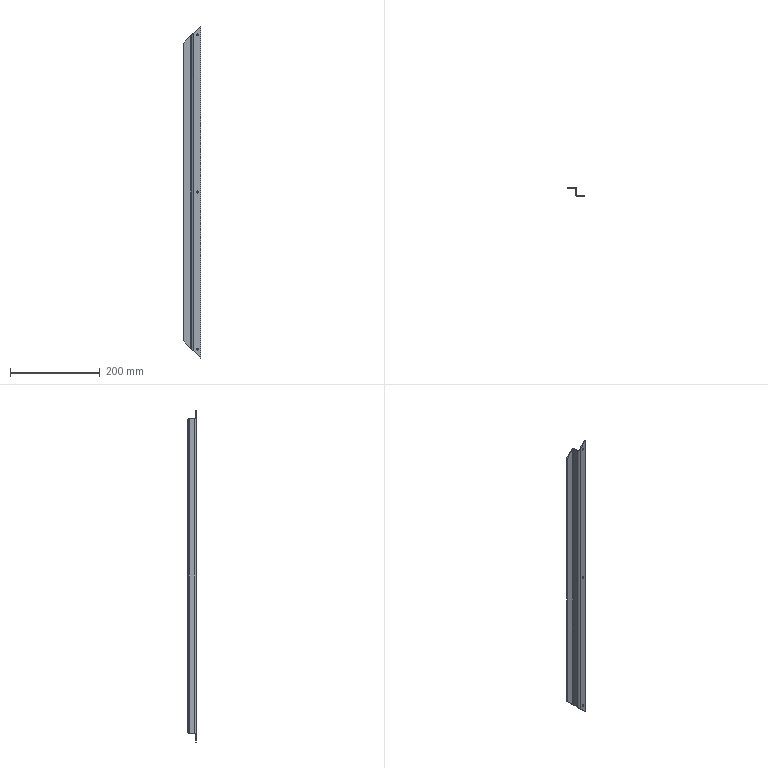Part | STEP file | SYL_0392D6J1SYL0380DJ100-463198 | 1 solid | 28 faces | box 38 x 20 x 740 mm | volume 74841 mm3 | plane 14 | cylinder 10 | spline 4 | commonest cylinder face diameters 4.5 x6 4 x2 8 x2